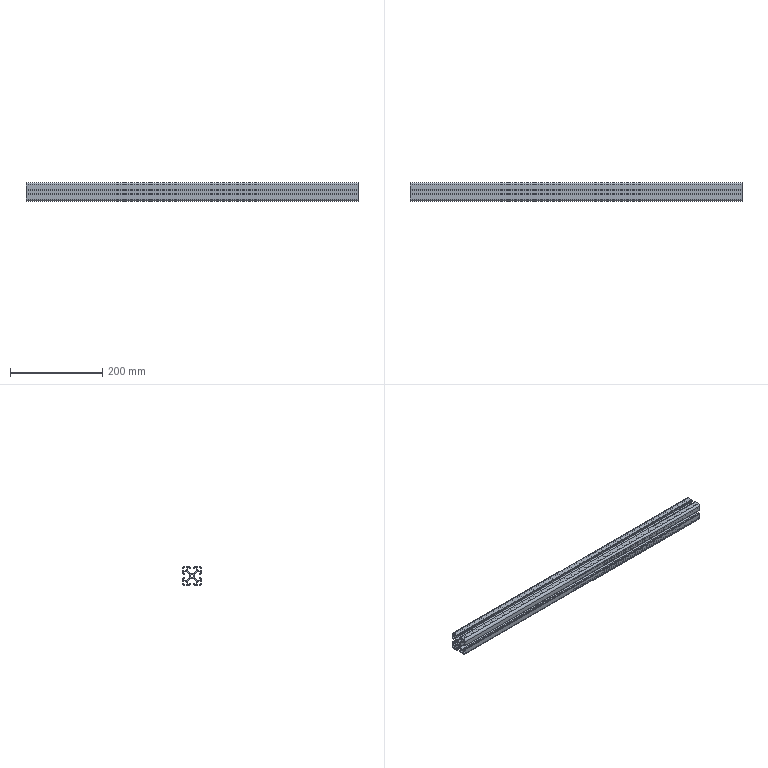Part | STEP file | MK-8-4040C-L-00 profile 4040C standard type 1270mm | 1 solid | 188 faces | box 720 x 40 x 40 mm | volume 346595 mm3 | cylinder 94 | plane 94 | commonest cylinder face diameters 0.6 x30 2 x28 4 x16 0.4 x8 6 x4 9 x4